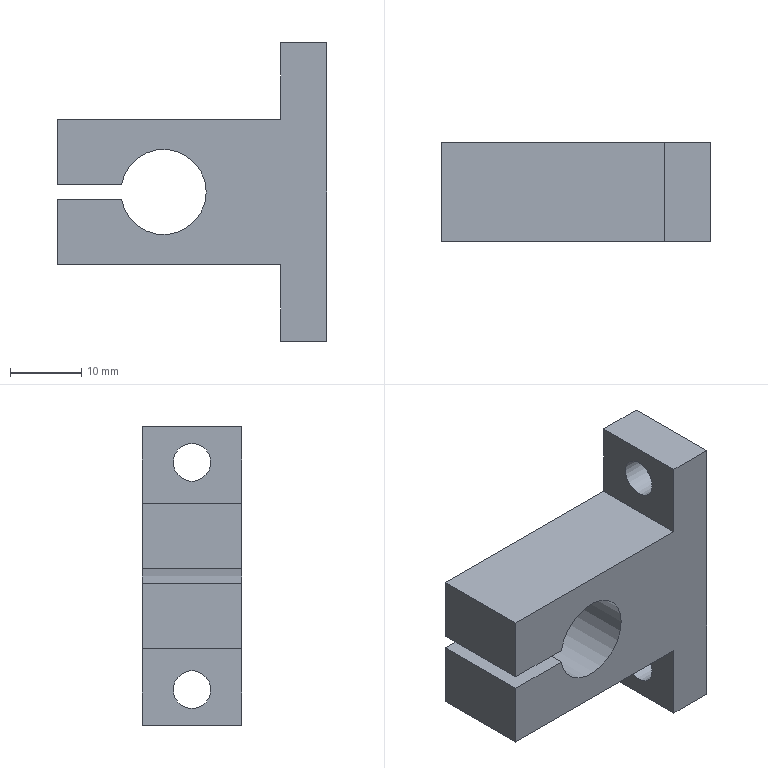Part | STEP file | 冲床-300配套压波_id278_x_t | 1 solid | 16 faces | box 38 x 14 x 42 mm | volume 10740 mm3 | plane 13 | cylinder 3 | commonest cylinder face diameters 5.3 x2 12 x1
STEP:
#1=CARTESIAN_POINT('',(1180.,-95.35,213.));
#2=VERTEX_POINT('',#1);
#3=CARTESIAN_POINT('',(1180.,-98.,213.));
#4=DIRECTION('',(-1.,0.,0.));
#5=DIRECTION('',(0.,1.,0.));
#6=AXIS2_PLACEMENT_3D('',#3,#4,#5);
#7=CIRCLE('',#6,2.65);
#8=EDGE_CURVE('',#2,#2,#7,.T.);
#9=ORIENTED_EDGE('',*,*,#8,.T.);
#10=EDGE_LOOP('',(#9));
#11=FACE_BOUND('',#10,.T.);
#12=CARTESIAN_POINT('',(1180.,-91.,208.));
#13=VERTEX_POINT('',#12);
#14=CARTESIAN_POINT('',(1180.,-91.,250.));
#15=VERTEX_POINT('',#14);
#16=CARTESIAN_POINT('',(1180.,-91.,208.));
#17=DIRECTION('',(0.,0.,1.));
#18=VECTOR('',#17,1.);
#19=LINE('',#16,#18);
#20=EDGE_CURVE('',#13,#15,#19,.T.);
#21=ORIENTED_EDGE('',*,*,#20,.T.);
#22=CARTESIAN_POINT('',(1180.,-105.,250.));
#23=VERTEX_POINT('',#22);
#24=CARTESIAN_POINT('',(1180.,-105.,250.));
#25=DIRECTION('',(0.,1.,0.));
#26=VECTOR('',#25,1.);
#27=LINE('',#24,#26);
#28=EDGE_CURVE('',#23,#15,#27,.T.);
#29=ORIENTED_EDGE('',*,*,#28,.F.);
#30=CARTESIAN_POINT('',(1180.,-105.,208.));
#31=VERTEX_POINT('',#30);
#32=CARTESIAN_POINT('',(1180.,-105.,229.));
#33=DIRECTION('',(0.,0.,1.));
#34=VECTOR('',#33,1.);
#35=LINE('',#32,#34);
#36=EDGE_CURVE('',#31,#23,#35,.T.);
#37=ORIENTED_EDGE('',*,*,#36,.F.);
#38=CARTESIAN_POINT('',(1180.,-105.,208.));
#39=DIRECTION('',(0.,1.,0.));
#40=VECTOR('',#39,1.);
#41=LINE('',#38,#40);
#42=EDGE_CURVE('',#31,#13,#41,.T.);
#43=ORIENTED_EDGE('',*,*,#42,.T.);
#44=EDGE_LOOP('',(#21,#29,#37,#43));
#45=FACE_BOUND('',#44,.T.);
#46=CARTESIAN_POINT('',(1180.,-95.35,245.));
#47=VERTEX_POINT('',#46);
#48=CARTESIAN_POINT('',(1180.,-98.,245.));
#49=DIRECTION('',(1.,0.,0.));
#50=DIRECTION('',(0.,1.,0.));
#51=AXIS2_PLACEMENT_3D('',#48,#49,#50);
#52=CIRCLE('',#51,2.65);
#53=EDGE_CURVE('',#47,#47,#52,.T.);
#54=ORIENTED_EDGE('',*,*,#53,.F.);
#55=EDGE_LOOP('',(#54));
#56=FACE_BOUND('',#55,.T.);
#57=CARTESIAN_POINT('',(1180.,-105.,208.));
#58=DIRECTION('',(-1.,0.,0.));
#59=DIRECTION('',(0.,1.,0.));
#60=AXIS2_PLACEMENT_3D('',#57,#58,#59);
#61=PLANE('',#60);
#62=ADVANCED_FACE('',(#11,#45,#56),#61,.F.);
#63=CARTESIAN_POINT('',(1142.,-105.,230.));
#64=VERTEX_POINT('',#63);
#65=CARTESIAN_POINT('',(1142.,-91.,230.));
#66=VERTEX_POINT('',#65);
#67=CARTESIAN_POINT('',(1142.,-105.,230.));
#68=DIRECTION('',(0.,1.,0.));
#69=VECTOR('',#68,1.);
#70=LINE('',#67,#69);
#71=EDGE_CURVE('',#64,#66,#70,.T.);
#72=ORIENTED_EDGE('',*,*,#71,.F.);
#73=CARTESIAN_POINT('',(1142.,-105.,239.25));
#74=VERTEX_POINT('',#73);
#75=CARTESIAN_POINT('',(1142.,-105.,239.25));
#76=DIRECTION('',(0.,0.,-1.));
#77=VECTOR('',#76,1.);
#78=LINE('',#75,#77);
#79=EDGE_CURVE('',#74,#64,#78,.T.);
#80=ORIENTED_EDGE('',*,*,#79,.F.);
#81=CARTESIAN_POINT('',(1142.,-91.,239.25));
#82=VERTEX_POINT('',#81);
#83=CARTESIAN_POINT('',(1142.,-105.,239.25));
#84=DIRECTION('',(0.,1.,0.));
#85=VECTOR('',#84,1.);
#86=LINE('',#83,#85);
#87=EDGE_CURVE('',#74,#82,#86,.T.);
#88=ORIENTED_EDGE('',*,*,#87,.T.);
#89=CARTESIAN_POINT('',(1142.,-91.,229.));
#90=DIRECTION('',(0.,0.,-1.));
#91=VECTOR('',#90,1.);
#92=LINE('',#89,#91);
#93=EDGE_CURVE('',#82,#66,#92,.T.);
#94=ORIENTED_EDGE('',*,*,#93,.T.);
#95=EDGE_LOOP('',(#72,#80,#88,#94));
#96=FACE_OUTER_BOUND('',#95,.T.);
#97=CARTESIAN_POINT('',(1142.,-105.,229.));
#98=DIRECTION('',(1.,0.,0.));
#99=DIRECTION('',(0.,-1.,0.));
#100=AXIS2_PLACEMENT_3D('',#97,#98,#99);
#101=PLANE('',#100);
#102=ADVANCED_FACE('',(#96),#101,.F.);
#103=CARTESIAN_POINT('',(1142.,-91.,228.));
#104=VERTEX_POINT('',#103);
#105=CARTESIAN_POINT('',(1142.,-105.,228.));
#106=VERTEX_POINT('',#105);
#107=CARTESIAN_POINT('',(1142.,-105.,228.));
#108=DIRECTION('',(0.,-1.,0.));
#109=VECTOR('',#108,1.);
#110=LINE('',#107,#109);
#111=EDGE_CURVE('',#104,#106,#110,.T.);
#112=ORIENTED_EDGE('',*,*,#111,.F.);
#113=CARTESIAN_POINT('',(1142.,-91.,218.75));
#114=VERTEX_POINT('',#113);
#115=CARTESIAN_POINT('',(1142.,-91.,229.));
#116=DIRECTION('',(0.,0.,-1.));
#117=VECTOR('',#116,1.);
#118=LINE('',#115,#117);
#119=EDGE_CURVE('',#104,#114,#118,.T.);
#120=ORIENTED_EDGE('',*,*,#119,.T.);
#121=CARTESIAN_POINT('',(1142.,-105.,218.75));
#122=VERTEX_POINT('',#121);
#123=CARTESIAN_POINT('',(1142.,-105.,218.75));
#124=DIRECTION('',(0.,1.,0.));
#125=VECTOR('',#124,1.);
#126=LINE('',#123,#125);
#127=EDGE_CURVE('',#122,#114,#126,.T.);
#128=ORIENTED_EDGE('',*,*,#127,.F.);
#129=CARTESIAN_POINT('',(1142.,-105.,239.25));
#130=DIRECTION('',(0.,0.,-1.));
#131=VECTOR('',#130,1.);
#132=LINE('',#129,#131);
#133=EDGE_CURVE('',#106,#122,#132,.T.);
#134=ORIENTED_EDGE('',*,*,#133,.F.);
#135=EDGE_LOOP('',(#112,#120,#128,#134));
#136=FACE_OUTER_BOUND('',#135,.T.);
#137=CARTESIAN_POINT('',(1142.,-105.,229.));
#138=DIRECTION('',(1.,0.,0.));
#139=DIRECTION('',(0.,-1.,0.));
#140=AXIS2_PLACEMENT_3D('',#137,#138,#139);
#141=PLANE('',#140);
#142=ADVANCED_FACE('',(#136),#141,.F.);
#143=CARTESIAN_POINT('',(1151.084,-105.,228.));
#144=VERTEX_POINT('',#143);
#145=CARTESIAN_POINT('',(1151.084,-105.,230.));
#146=VERTEX_POINT('',#145);
#147=CARTESIAN_POINT('',(1157.,-105.,229.));
#148=DIRECTION('',(0.,-1.,0.));
#149=DIRECTION('',(0.,0.,-1.));
#150=AXIS2_PLACEMENT_3D('',#147,#148,#149);
#151=CIRCLE('',#150,6.);
#152=EDGE_CURVE('',#144,#146,#151,.T.);
#153=ORIENTED_EDGE('',*,*,#152,.T.);
#154=CARTESIAN_POINT('',(1151.084,-91.,230.));
#155=VERTEX_POINT('',#154);
#156=CARTESIAN_POINT('',(1151.084,-105.,230.));
#157=DIRECTION('',(0.,1.,0.));
#158=VECTOR('',#157,1.);
#159=LINE('',#156,#158);
#160=EDGE_CURVE('',#146,#155,#159,.T.);
#161=ORIENTED_EDGE('',*,*,#160,.T.);
#162=CARTESIAN_POINT('',(1151.084,-91.,228.));
#163=VERTEX_POINT('',#162);
#164=CARTESIAN_POINT('',(1157.,-91.,229.));
#165=DIRECTION('',(0.,-1.,0.));
#166=DIRECTION('',(0.,0.,-1.));
#167=AXIS2_PLACEMENT_3D('',#164,#165,#166);
#168=CIRCLE('',#167,6.);
#169=EDGE_CURVE('',#163,#155,#168,.T.);
#170=ORIENTED_EDGE('',*,*,#169,.F.);
#171=CARTESIAN_POINT('',(1151.084,-105.,228.));
#172=DIRECTION('',(0.,-1.,0.));
#173=VECTOR('',#172,1.);
#174=LINE('',#171,#173);
#175=EDGE_CURVE('',#163,#144,#174,.T.);
#176=ORIENTED_EDGE('',*,*,#175,.T.);
#177=EDGE_LOOP('',(#153,#161,#170,#176));
#178=FACE_OUTER_BOUND('',#177,.T.);
#179=CARTESIAN_POINT('',(1157.,-105.,229.));
#180=DIRECTION('',(0.,1.,0.));
#181=DIRECTION('',(1.,0.,0.));
#182=AXIS2_PLACEMENT_3D('',#179,#180,#181);
#183=CYLINDRICAL_SURFACE('',#182,6.);
#184=ADVANCED_FACE('',(#178),#183,.F.);
#185=ORIENTED_EDGE('',*,*,#79,.T.);
#186=CARTESIAN_POINT('',(1157.,-105.,230.));
#187=DIRECTION('',(1.,0.,0.));
#188=VECTOR('',#187,1.);
#189=LINE('',#186,#188);
#190=EDGE_CURVE('',#64,#146,#189,.T.);
#191=ORIENTED_EDGE('',*,*,#190,.T.);
#192=ORIENTED_EDGE('',*,*,#152,.F.);
#193=CARTESIAN_POINT('',(1157.,-105.,228.));
#194=DIRECTION('',(-1.,0.,0.));
#195=VECTOR('',#194,1.);
#196=LINE('',#193,#195);
#197=EDGE_CURVE('',#144,#106,#196,.T.);
#198=ORIENTED_EDGE('',*,*,#197,.T.);
#199=ORIENTED_EDGE('',*,*,#133,.T.);
#200=CARTESIAN_POINT('',(1173.5,-105.,218.75));
#201=VERTEX_POINT('',#200);
#202=CARTESIAN_POINT('',(1142.,-105.,218.75));
#203=DIRECTION('',(1.,0.,0.));
#204=VECTOR('',#203,1.);
#205=LINE('',#202,#204);
#206=EDGE_CURVE('',#122,#201,#205,.T.);
#207=ORIENTED_EDGE('',*,*,#206,.T.);
#208=CARTESIAN_POINT('',(1173.5,-105.,208.));
#209=VERTEX_POINT('',#208);
#210=CARTESIAN_POINT('',(1173.5,-105.,218.75));
#211=DIRECTION('',(0.,0.,-1.));
#212=VECTOR('',#211,1.);
#213=LINE('',#210,#212);
#214=EDGE_CURVE('',#201,#209,#213,.T.);
#215=ORIENTED_EDGE('',*,*,#214,.T.);
#216=CARTESIAN_POINT('',(1173.5,-105.,208.));
#217=DIRECTION('',(1.,0.,0.));
#218=VECTOR('',#217,1.);
#219=LINE('',#216,#218);
#220=EDGE_CURVE('',#209,#31,#219,.T.);
#221=ORIENTED_EDGE('',*,*,#220,.T.);
#222=ORIENTED_EDGE('',*,*,#36,.T.);
#223=CARTESIAN_POINT('',(1173.5,-105.,250.));
#224=VERTEX_POINT('',#223);
#225=CARTESIAN_POINT('',(1180.,-105.,250.));
#226=DIRECTION('',(-1.,0.,0.));
#227=VECTOR('',#226,1.);
#228=LINE('',#225,#227);
#229=EDGE_CURVE('',#23,#224,#228,.T.);
#230=ORIENTED_EDGE('',*,*,#229,.T.);
#231=CARTESIAN_POINT('',(1173.5,-105.,239.25));
#232=VERTEX_POINT('',#231);
#233=CARTESIAN_POINT('',(1173.5,-105.,250.));
#234=DIRECTION('',(0.,0.,-1.));
#235=VECTOR('',#234,1.);
#236=LINE('',#233,#235);
#237=EDGE_CURVE('',#224,#232,#236,.T.);
#238=ORIENTED_EDGE('',*,*,#237,.T.);
#239=CARTESIAN_POINT('',(1173.5,-105.,239.25));
#240=DIRECTION('',(-1.,0.,0.));
#241=VECTOR('',#240,1.);
#242=LINE('',#239,#241);
#243=EDGE_CURVE('',#232,#74,#242,.T.);
#244=ORIENTED_EDGE('',*,*,#243,.T.);
#245=EDGE_LOOP('',(#185,#191,#192,#198,#199,#207,#215,#221,#222,#230,#238,#244));
#246=FACE_OUTER_BOUND('',#245,.T.);
#247=CARTESIAN_POINT('',(1157.,-105.,229.));
#248=DIRECTION('',(0.,-1.,0.));
#249=DIRECTION('',(-1.,0.,0.));
#250=AXIS2_PLACEMENT_3D('',#247,#248,#249);
#251=PLANE('',#250);
#252=ADVANCED_FACE('',(#246),#251,.T.);
#253=CARTESIAN_POINT('',(1157.,-91.,230.));
#254=DIRECTION('',(1.,0.,0.));
#255=VECTOR('',#254,1.);
#256=LINE('',#253,#255);
#257=EDGE_CURVE('',#66,#155,#256,.T.);
#258=ORIENTED_EDGE('',*,*,#257,.F.);
#259=ORIENTED_EDGE('',*,*,#93,.F.);
#260=CARTESIAN_POINT('',(1173.5,-91.,239.25));
#261=VERTEX_POINT('',#260);
#262=CARTESIAN_POINT('',(1173.5,-91.,239.25));
#263=DIRECTION('',(-1.,0.,0.));
#264=VECTOR('',#263,1.);
#265=LINE('',#262,#264);
#266=EDGE_CURVE('',#261,#82,#265,.T.);
#267=ORIENTED_EDGE('',*,*,#266,.F.);
#268=CARTESIAN_POINT('',(1173.5,-91.,250.));
#269=VERTEX_POINT('',#268);
#270=CARTESIAN_POINT('',(1173.5,-91.,250.));
#271=DIRECTION('',(0.,0.,-1.));
#272=VECTOR('',#271,1.);
#273=LINE('',#270,#272);
#274=EDGE_CURVE('',#269,#261,#273,.T.);
#275=ORIENTED_EDGE('',*,*,#274,.F.);
#276=CARTESIAN_POINT('',(1180.,-91.,250.));
#277=DIRECTION('',(-1.,0.,0.));
#278=VECTOR('',#277,1.);
#279=LINE('',#276,#278);
#280=EDGE_CURVE('',#15,#269,#279,.T.);
#281=ORIENTED_EDGE('',*,*,#280,.F.);
#282=ORIENTED_EDGE('',*,*,#20,.F.);
#283=CARTESIAN_POINT('',(1173.5,-91.,208.));
#284=VERTEX_POINT('',#283);
#285=CARTESIAN_POINT('',(1173.5,-91.,208.));
#286=DIRECTION('',(1.,0.,0.));
#287=VECTOR('',#286,1.);
#288=LINE('',#285,#287);
#289=EDGE_CURVE('',#284,#13,#288,.T.);
#290=ORIENTED_EDGE('',*,*,#289,.F.);
#291=CARTESIAN_POINT('',(1173.5,-91.,218.75));
#292=VERTEX_POINT('',#291);
#293=CARTESIAN_POINT('',(1173.5,-91.,218.75));
#294=DIRECTION('',(0.,0.,-1.));
#295=VECTOR('',#294,1.);
#296=LINE('',#293,#295);
#297=EDGE_CURVE('',#292,#284,#296,.T.);
#298=ORIENTED_EDGE('',*,*,#297,.F.);
#299=CARTESIAN_POINT('',(1142.,-91.,218.75));
#300=DIRECTION('',(1.,0.,0.));
#301=VECTOR('',#300,1.);
#302=LINE('',#299,#301);
#303=EDGE_CURVE('',#114,#292,#302,.T.);
#304=ORIENTED_EDGE('',*,*,#303,.F.);
#305=ORIENTED_EDGE('',*,*,#119,.F.);
#306=CARTESIAN_POINT('',(1157.,-91.,228.));
#307=DIRECTION('',(-1.,0.,0.));
#308=VECTOR('',#307,1.);
#309=LINE('',#306,#308);
#310=EDGE_CURVE('',#163,#104,#309,.T.);
#311=ORIENTED_EDGE('',*,*,#310,.F.);
#312=ORIENTED_EDGE('',*,*,#169,.T.);
#313=EDGE_LOOP('',(#258,#259,#267,#275,#281,#282,#290,#298,#304,#305,#311,#312));
#314=FACE_OUTER_BOUND('',#313,.T.);
#315=CARTESIAN_POINT('',(1157.,-91.,229.));
#316=DIRECTION('',(0.,-1.,0.));
#317=DIRECTION('',(-1.,0.,0.));
#318=AXIS2_PLACEMENT_3D('',#315,#316,#317);
#319=PLANE('',#318);
#320=ADVANCED_FACE('',(#314),#319,.F.);
#321=ORIENTED_EDGE('',*,*,#280,.T.);
#322=CARTESIAN_POINT('',(1173.5,-105.,250.));
#323=DIRECTION('',(0.,1.,0.));
#324=VECTOR('',#323,1.);
#325=LINE('',#322,#324);
#326=EDGE_CURVE('',#224,#269,#325,.T.);
#327=ORIENTED_EDGE('',*,*,#326,.F.);
#328=ORIENTED_EDGE('',*,*,#229,.F.);
#329=ORIENTED_EDGE('',*,*,#28,.T.);
#330=EDGE_LOOP('',(#321,#327,#328,#329));
#331=FACE_OUTER_BOUND('',#330,.T.);
#332=CARTESIAN_POINT('',(1180.,-105.,250.));
#333=DIRECTION('',(0.,0.,-1.));
#334=DIRECTION('',(1.,0.,0.));
#335=AXIS2_PLACEMENT_3D('',#332,#333,#334);
#336=PLANE('',#335);
#337=ADVANCED_FACE('',(#331),#336,.F.);
#338=CARTESIAN_POINT('',(1173.5,-100.65,245.));
#339=VERTEX_POINT('',#338);
#340=CARTESIAN_POINT('',(1173.5,-98.,245.));
#341=DIRECTION('',(-1.,0.,0.));
#342=DIRECTION('',(0.,-1.,0.));
#343=AXIS2_PLACEMENT_3D('',#340,#341,#342);
#344=CIRCLE('',#343,2.65);
#345=EDGE_CURVE('',#339,#339,#344,.T.);
#346=ORIENTED_EDGE('',*,*,#345,.F.);
#347=EDGE_LOOP('',(#346));
#348=FACE_BOUND('',#347,.T.);
#349=ORIENTED_EDGE('',*,*,#274,.T.);
#350=CARTESIAN_POINT('',(1173.5,-105.,239.25));
#351=DIRECTION('',(0.,1.,0.));
#352=VECTOR('',#351,1.);
#353=LINE('',#350,#352);
#354=EDGE_CURVE('',#232,#261,#353,.T.);
#355=ORIENTED_EDGE('',*,*,#354,.F.);
#356=ORIENTED_EDGE('',*,*,#237,.F.);
#357=ORIENTED_EDGE('',*,*,#326,.T.);
#358=EDGE_LOOP('',(#349,#355,#356,#357));
#359=FACE_BOUND('',#358,.T.);
#360=CARTESIAN_POINT('',(1173.5,-105.,250.));
#361=DIRECTION('',(1.,0.,0.));
#362=DIRECTION('',(0.,-1.,0.));
#363=AXIS2_PLACEMENT_3D('',#360,#361,#362);
#364=PLANE('',#363);
#365=ADVANCED_FACE('',(#348,#359),#364,.F.);
#366=ORIENTED_EDGE('',*,*,#266,.T.);
#367=ORIENTED_EDGE('',*,*,#87,.F.);
#368=ORIENTED_EDGE('',*,*,#243,.F.);
#369=ORIENTED_EDGE('',*,*,#354,.T.);
#370=EDGE_LOOP('',(#366,#367,#368,#369));
#371=FACE_OUTER_BOUND('',#370,.T.);
#372=CARTESIAN_POINT('',(1173.5,-105.,239.25));
#373=DIRECTION('',(0.,0.,-1.));
#374=DIRECTION('',(0.,-1.,0.));
#375=AXIS2_PLACEMENT_3D('',#372,#373,#374);
#376=PLANE('',#375);
#377=ADVANCED_FACE('',(#371),#376,.F.);
#378=ORIENTED_EDGE('',*,*,#303,.T.);
#379=CARTESIAN_POINT('',(1173.5,-105.,218.75));
#380=DIRECTION('',(0.,1.,0.));
#381=VECTOR('',#380,1.);
#382=LINE('',#379,#381);
#383=EDGE_CURVE('',#201,#292,#382,.T.);
#384=ORIENTED_EDGE('',*,*,#383,.F.);
#385=ORIENTED_EDGE('',*,*,#206,.F.);
#386=ORIENTED_EDGE('',*,*,#127,.T.);
#387=EDGE_LOOP('',(#378,#384,#385,#386));
#388=FACE_OUTER_BOUND('',#387,.T.);
#389=CARTESIAN_POINT('',(1142.,-105.,218.75));
#390=DIRECTION('',(0.,0.,1.));
#391=DIRECTION('',(0.,1.,0.));
#392=AXIS2_PLACEMENT_3D('',#389,#390,#391);
#393=PLANE('',#392);
#394=ADVANCED_FACE('',(#388),#393,.F.);
#395=CARTESIAN_POINT('',(1173.5,-100.65,213.));
#396=VERTEX_POINT('',#395);
#397=CARTESIAN_POINT('',(1173.5,-98.,213.));
#398=DIRECTION('',(1.,0.,0.));
#399=DIRECTION('',(0.,-1.,0.));
#400=AXIS2_PLACEMENT_3D('',#397,#398,#399);
#401=CIRCLE('',#400,2.65);
#402=EDGE_CURVE('',#396,#396,#401,.T.);
#403=ORIENTED_EDGE('',*,*,#402,.T.);
#404=EDGE_LOOP('',(#403));
#405=FACE_BOUND('',#404,.T.);
#406=ORIENTED_EDGE('',*,*,#297,.T.);
#407=CARTESIAN_POINT('',(1173.5,-105.,208.));
#408=DIRECTION('',(0.,1.,0.));
#409=VECTOR('',#408,1.);
#410=LINE('',#407,#409);
#411=EDGE_CURVE('',#209,#284,#410,.T.);
#412=ORIENTED_EDGE('',*,*,#411,.F.);
#413=ORIENTED_EDGE('',*,*,#214,.F.);
#414=ORIENTED_EDGE('',*,*,#383,.T.);
#415=EDGE_LOOP('',(#406,#412,#413,#414));
#416=FACE_BOUND('',#415,.T.);
#417=CARTESIAN_POINT('',(1173.5,-105.,218.75));
#418=DIRECTION('',(1.,0.,0.));
#419=DIRECTION('',(0.,-1.,0.));
#420=AXIS2_PLACEMENT_3D('',#417,#418,#419);
#421=PLANE('',#420);
#422=ADVANCED_FACE('',(#405,#416),#421,.F.);
#423=ORIENTED_EDGE('',*,*,#289,.T.);
#424=ORIENTED_EDGE('',*,*,#42,.F.);
#425=ORIENTED_EDGE('',*,*,#220,.F.);
#426=ORIENTED_EDGE('',*,*,#411,.T.);
#427=EDGE_LOOP('',(#423,#424,#425,#426));
#428=FACE_OUTER_BOUND('',#427,.T.);
#429=CARTESIAN_POINT('',(1173.5,-105.,208.));
#430=DIRECTION('',(0.,0.,1.));
#431=DIRECTION('',(-1.,0.,0.));
#432=AXIS2_PLACEMENT_3D('',#429,#430,#431);
#433=PLANE('',#432);
#434=ADVANCED_FACE('',(#428),#433,.F.);
#435=ORIENTED_EDGE('',*,*,#175,.F.);
#436=ORIENTED_EDGE('',*,*,#310,.T.);
#437=ORIENTED_EDGE('',*,*,#111,.T.);
#438=ORIENTED_EDGE('',*,*,#197,.F.);
#439=EDGE_LOOP('',(#435,#436,#437,#438));
#440=FACE_OUTER_BOUND('',#439,.T.);
#441=CARTESIAN_POINT('',(1136.419,-119.,228.));
#442=DIRECTION('',(0.,0.,1.));
#443=DIRECTION('',(0.,1.,0.));
#444=AXIS2_PLACEMENT_3D('',#441,#442,#443);
#445=PLANE('',#444);
#446=ADVANCED_FACE('',(#440),#445,.T.);
#447=ORIENTED_EDGE('',*,*,#71,.T.);
#448=ORIENTED_EDGE('',*,*,#257,.T.);
#449=ORIENTED_EDGE('',*,*,#160,.F.);
#450=ORIENTED_EDGE('',*,*,#190,.F.);
#451=EDGE_LOOP('',(#447,#448,#449,#450));
#452=FACE_OUTER_BOUND('',#451,.T.);
#453=CARTESIAN_POINT('',(1155.8,-119.,230.));
#454=DIRECTION('',(0.,0.,-1.));
#455=DIRECTION('',(0.,-1.,0.));
#456=AXIS2_PLACEMENT_3D('',#453,#454,#455);
#457=PLANE('',#456);
#458=ADVANCED_FACE('',(#452),#457,.T.);
#459=ORIENTED_EDGE('',*,*,#8,.F.);
#460=EDGE_LOOP('',(#459));
#461=FACE_BOUND('',#460,.T.);
#462=ORIENTED_EDGE('',*,*,#402,.F.);
#463=EDGE_LOOP('',(#462));
#464=FACE_BOUND('',#463,.T.);
#465=CARTESIAN_POINT('',(1159.5,-98.,213.));
#466=DIRECTION('',(1.,0.,0.));
#467=DIRECTION('',(0.,-1.,0.));
#468=AXIS2_PLACEMENT_3D('',#465,#466,#467);
#469=CYLINDRICAL_SURFACE('',#468,2.65);
#470=ADVANCED_FACE('',(#461,#464),#469,.F.);
#471=ORIENTED_EDGE('',*,*,#53,.T.);
#472=EDGE_LOOP('',(#471));
#473=FACE_BOUND('',#472,.T.);
#474=ORIENTED_EDGE('',*,*,#345,.T.);
#475=EDGE_LOOP('',(#474));
#476=FACE_BOUND('',#475,.T.);
#477=CARTESIAN_POINT('',(1159.5,-98.,245.));
#478=DIRECTION('',(1.,0.,0.));
#479=DIRECTION('',(0.,-1.,0.));
#480=AXIS2_PLACEMENT_3D('',#477,#478,#479);
#481=CYLINDRICAL_SURFACE('',#480,2.65);
#482=ADVANCED_FACE('',(#473,#476),#481,.F.);
#483=CLOSED_SHELL('',(#62,#102,#142,#184,#252,#320,#337,#365,#377,#394,#422,#434,#446,#458,#470,#482));
#484=MANIFOLD_SOLID_BREP('',#483);
#485=(LENGTH_UNIT()NAMED_UNIT(*)SI_UNIT(.MILLI.,.METRE.));
#486=UNCERTAINTY_MEASURE_WITH_UNIT(LENGTH_MEASURE(0.00002),#485,'','');
#487=(NAMED_UNIT(*)PLANE_ANGLE_UNIT()SI_UNIT($,.RADIAN.));
#488=PLANE_ANGLE_MEASURE_WITH_UNIT(PLANE_ANGLE_MEASURE(0.01745),#487);
#489=DIMENSIONAL_EXPONENTS(0.,0.,0.,0.,0.,0.,0.);
#490=(CONVERSION_BASED_UNIT('DEGREE',#488)NAMED_UNIT(#489)PLANE_ANGLE_UNIT());
#491=(NAMED_UNIT(*)SI_UNIT($,.STERADIAN.)SOLID_ANGLE_UNIT());
#492=(GEOMETRIC_REPRESENTATION_CONTEXT(3)GLOBAL_UNCERTAINTY_ASSIGNED_CONTEXT((#486))GLOBAL_UNIT_ASSIGNED_CONTEXT((#485,#490,#491))REPRESENTATION_CONTEXT('',''));
#493=ADVANCED_BREP_SHAPE_REPRESENTATION('',(#484),#492);